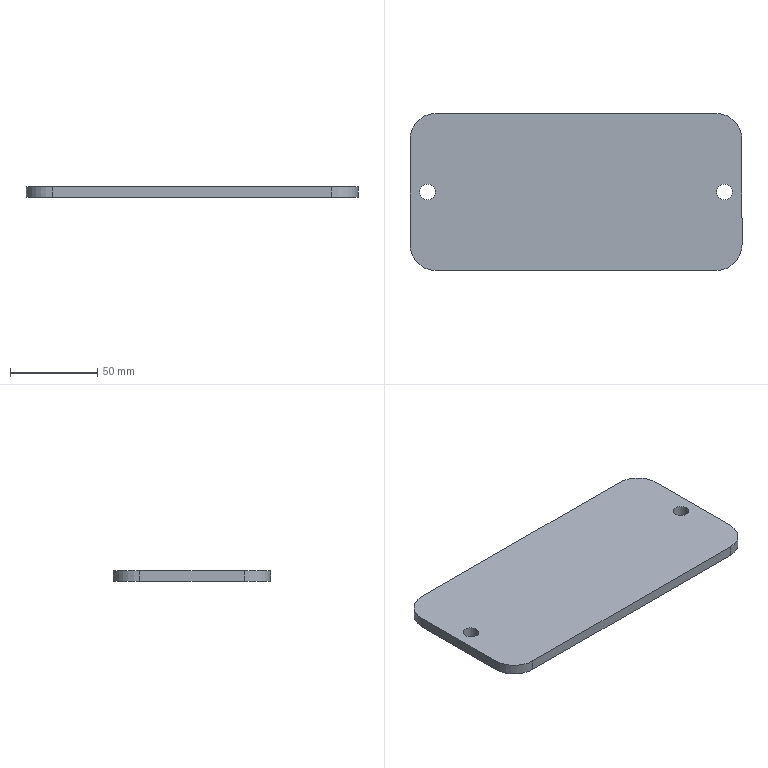Part | SolidWorks | features FlatPattern 1, SMBaseFlange 1, SheetMetal 1 | 1 solid | 14 faces | box 190 x 90 x 6 mm | volume 100678 mm3 | cylinder 8 | plane 6 | commonest cylinder face diameters 9 x4 30 x4
STEP:
#1=CARTESIAN_POINT('',(175.5,45.,-6.));
#2=VERTEX_POINT('',#1);
#3=CARTESIAN_POINT('',(184.5,45.,-6.));
#4=VERTEX_POINT('',#3);
#5=CARTESIAN_POINT('',(180.,45.,-6.));
#6=DIRECTION('',(0.,0.,1.));
#7=DIRECTION('',(1.,0.,0.));
#8=AXIS2_PLACEMENT_3D('',#5,#6,#7);
#9=CIRCLE('',#8,4.5);
#10=EDGE_CURVE('',#2,#4,#9,.T.);
#11=ORIENTED_EDGE('',*,*,#10,.F.);
#12=CARTESIAN_POINT('',(175.5,45.,0.));
#13=VERTEX_POINT('',#12);
#14=CARTESIAN_POINT('',(175.5,45.,-6.));
#15=DIRECTION('',(0.,0.,1.));
#16=VECTOR('',#15,1000.);
#17=LINE('',#14,#16);
#18=EDGE_CURVE('',#2,#13,#17,.T.);
#19=ORIENTED_EDGE('',*,*,#18,.T.);
#20=CARTESIAN_POINT('',(184.5,45.,0.));
#21=VERTEX_POINT('',#20);
#22=CARTESIAN_POINT('',(180.,45.,0.));
#23=DIRECTION('',(0.,0.,1.));
#24=DIRECTION('',(1.,0.,0.));
#25=AXIS2_PLACEMENT_3D('',#22,#23,#24);
#26=CIRCLE('',#25,4.5);
#27=EDGE_CURVE('',#13,#21,#26,.T.);
#28=ORIENTED_EDGE('',*,*,#27,.T.);
#29=CARTESIAN_POINT('',(184.5,45.,-6.));
#30=DIRECTION('',(0.,0.,1.));
#31=VECTOR('',#30,1000.);
#32=LINE('',#29,#31);
#33=EDGE_CURVE('',#4,#21,#32,.T.);
#34=ORIENTED_EDGE('',*,*,#33,.F.);
#35=EDGE_LOOP('',(#11,#19,#28,#34));
#36=FACE_OUTER_BOUND('',#35,.T.);
#37=CARTESIAN_POINT('',(180.,45.,-6.));
#38=DIRECTION('',(0.,0.,1.));
#39=DIRECTION('',(1.,0.,0.));
#40=AXIS2_PLACEMENT_3D('',#37,#38,#39);
#41=CYLINDRICAL_SURFACE('',#40,4.5);
#42=ADVANCED_FACE('',(#36),#41,.F.);
#43=CARTESIAN_POINT('',(5.5,45.,-6.));
#44=VERTEX_POINT('',#43);
#45=CARTESIAN_POINT('',(14.5,45.,-6.));
#46=VERTEX_POINT('',#45);
#47=CARTESIAN_POINT('',(10.,45.,-6.));
#48=DIRECTION('',(0.,0.,1.));
#49=DIRECTION('',(1.,0.,0.));
#50=AXIS2_PLACEMENT_3D('',#47,#48,#49);
#51=CIRCLE('',#50,4.5);
#52=EDGE_CURVE('',#44,#46,#51,.T.);
#53=ORIENTED_EDGE('',*,*,#52,.F.);
#54=CARTESIAN_POINT('',(5.5,45.,0.));
#55=VERTEX_POINT('',#54);
#56=CARTESIAN_POINT('',(5.5,45.,-6.));
#57=DIRECTION('',(0.,0.,1.));
#58=VECTOR('',#57,1000.);
#59=LINE('',#56,#58);
#60=EDGE_CURVE('',#44,#55,#59,.T.);
#61=ORIENTED_EDGE('',*,*,#60,.T.);
#62=CARTESIAN_POINT('',(14.5,45.,0.));
#63=VERTEX_POINT('',#62);
#64=CARTESIAN_POINT('',(10.,45.,0.));
#65=DIRECTION('',(0.,0.,1.));
#66=DIRECTION('',(1.,0.,0.));
#67=AXIS2_PLACEMENT_3D('',#64,#65,#66);
#68=CIRCLE('',#67,4.5);
#69=EDGE_CURVE('',#55,#63,#68,.T.);
#70=ORIENTED_EDGE('',*,*,#69,.T.);
#71=CARTESIAN_POINT('',(14.5,45.,-6.));
#72=DIRECTION('',(0.,0.,1.));
#73=VECTOR('',#72,1000.);
#74=LINE('',#71,#73);
#75=EDGE_CURVE('',#46,#63,#74,.T.);
#76=ORIENTED_EDGE('',*,*,#75,.F.);
#77=EDGE_LOOP('',(#53,#61,#70,#76));
#78=FACE_OUTER_BOUND('',#77,.T.);
#79=CARTESIAN_POINT('',(10.,45.,-6.));
#80=DIRECTION('',(0.,0.,1.));
#81=DIRECTION('',(1.,0.,0.));
#82=AXIS2_PLACEMENT_3D('',#79,#80,#81);
#83=CYLINDRICAL_SURFACE('',#82,4.5);
#84=ADVANCED_FACE('',(#78),#83,.F.);
#85=CARTESIAN_POINT('',(175.,0.,0.));
#86=VERTEX_POINT('',#85);
#87=CARTESIAN_POINT('',(190.,15.,0.));
#88=VERTEX_POINT('',#87);
#89=CARTESIAN_POINT('',(175.,15.,0.));
#90=DIRECTION('',(0.,0.,1.));
#91=DIRECTION('',(-1.,0.,0.));
#92=AXIS2_PLACEMENT_3D('',#89,#90,#91);
#93=CIRCLE('',#92,15.);
#94=EDGE_CURVE('',#86,#88,#93,.T.);
#95=ORIENTED_EDGE('',*,*,#94,.F.);
#96=CARTESIAN_POINT('',(175.,0.,-6.));
#97=VERTEX_POINT('',#96);
#98=CARTESIAN_POINT('',(175.,0.,-6.));
#99=DIRECTION('',(0.,0.,1.));
#100=VECTOR('',#99,1000.);
#101=LINE('',#98,#100);
#102=EDGE_CURVE('',#97,#86,#101,.T.);
#103=ORIENTED_EDGE('',*,*,#102,.F.);
#104=CARTESIAN_POINT('',(190.,15.,-6.));
#105=VERTEX_POINT('',#104);
#106=CARTESIAN_POINT('',(175.,15.,-6.));
#107=DIRECTION('',(0.,0.,1.));
#108=DIRECTION('',(-1.,0.,0.));
#109=AXIS2_PLACEMENT_3D('',#106,#107,#108);
#110=CIRCLE('',#109,15.);
#111=EDGE_CURVE('',#97,#105,#110,.T.);
#112=ORIENTED_EDGE('',*,*,#111,.T.);
#113=CARTESIAN_POINT('',(190.,15.,-6.));
#114=DIRECTION('',(0.,0.,1.));
#115=VECTOR('',#114,1000.);
#116=LINE('',#113,#115);
#117=EDGE_CURVE('',#105,#88,#116,.T.);
#118=ORIENTED_EDGE('',*,*,#117,.T.);
#119=EDGE_LOOP('',(#95,#103,#112,#118));
#120=FACE_OUTER_BOUND('',#119,.T.);
#121=CARTESIAN_POINT('',(175.,15.,-6.));
#122=DIRECTION('',(0.,0.,1.));
#123=DIRECTION('',(1.,0.,0.));
#124=AXIS2_PLACEMENT_3D('',#121,#122,#123);
#125=CYLINDRICAL_SURFACE('',#124,15.);
#126=ADVANCED_FACE('',(#120),#125,.T.);
#127=CARTESIAN_POINT('',(15.,0.,0.));
#128=VERTEX_POINT('',#127);
#129=CARTESIAN_POINT('',(15.,0.,0.));
#130=DIRECTION('',(1.,0.,0.));
#131=VECTOR('',#130,1000.);
#132=LINE('',#129,#131);
#133=EDGE_CURVE('',#128,#86,#132,.T.);
#134=ORIENTED_EDGE('',*,*,#133,.F.);
#135=CARTESIAN_POINT('',(15.,0.,-6.));
#136=VERTEX_POINT('',#135);
#137=CARTESIAN_POINT('',(15.,0.,-6.));
#138=DIRECTION('',(0.,0.,1.));
#139=VECTOR('',#138,1000.);
#140=LINE('',#137,#139);
#141=EDGE_CURVE('',#136,#128,#140,.T.);
#142=ORIENTED_EDGE('',*,*,#141,.F.);
#143=CARTESIAN_POINT('',(15.,0.,-6.));
#144=DIRECTION('',(1.,0.,0.));
#145=VECTOR('',#144,1000.);
#146=LINE('',#143,#145);
#147=EDGE_CURVE('',#136,#97,#146,.T.);
#148=ORIENTED_EDGE('',*,*,#147,.T.);
#149=ORIENTED_EDGE('',*,*,#102,.T.);
#150=EDGE_LOOP('',(#134,#142,#148,#149));
#151=FACE_OUTER_BOUND('',#150,.T.);
#152=CARTESIAN_POINT('',(15.,0.,-6.));
#153=DIRECTION('',(0.,-1.,0.));
#154=DIRECTION('',(0.,0.,-1.));
#155=AXIS2_PLACEMENT_3D('',#152,#153,#154);
#156=PLANE('',#155);
#157=ADVANCED_FACE('',(#151),#156,.T.);
#158=CARTESIAN_POINT('',(0.,15.,0.));
#159=VERTEX_POINT('',#158);
#160=CARTESIAN_POINT('',(15.,15.,0.));
#161=DIRECTION('',(0.,0.,1.));
#162=DIRECTION('',(-1.,0.,0.));
#163=AXIS2_PLACEMENT_3D('',#160,#161,#162);
#164=CIRCLE('',#163,15.);
#165=EDGE_CURVE('',#159,#128,#164,.T.);
#166=ORIENTED_EDGE('',*,*,#165,.F.);
#167=CARTESIAN_POINT('',(0.,15.,-6.));
#168=VERTEX_POINT('',#167);
#169=CARTESIAN_POINT('',(0.,15.,-6.));
#170=DIRECTION('',(0.,0.,1.));
#171=VECTOR('',#170,1000.);
#172=LINE('',#169,#171);
#173=EDGE_CURVE('',#168,#159,#172,.T.);
#174=ORIENTED_EDGE('',*,*,#173,.F.);
#175=CARTESIAN_POINT('',(15.,15.,-6.));
#176=DIRECTION('',(0.,0.,1.));
#177=DIRECTION('',(-1.,0.,0.));
#178=AXIS2_PLACEMENT_3D('',#175,#176,#177);
#179=CIRCLE('',#178,15.);
#180=EDGE_CURVE('',#168,#136,#179,.T.);
#181=ORIENTED_EDGE('',*,*,#180,.T.);
#182=ORIENTED_EDGE('',*,*,#141,.T.);
#183=EDGE_LOOP('',(#166,#174,#181,#182));
#184=FACE_OUTER_BOUND('',#183,.T.);
#185=CARTESIAN_POINT('',(15.,15.,-6.));
#186=DIRECTION('',(0.,0.,1.));
#187=DIRECTION('',(1.,0.,0.));
#188=AXIS2_PLACEMENT_3D('',#185,#186,#187);
#189=CYLINDRICAL_SURFACE('',#188,15.);
#190=ADVANCED_FACE('',(#184),#189,.T.);
#191=CARTESIAN_POINT('',(0.,75.,0.));
#192=VERTEX_POINT('',#191);
#193=CARTESIAN_POINT('',(0.,15.,0.));
#194=DIRECTION('',(0.,-1.,0.));
#195=VECTOR('',#194,1000.);
#196=LINE('',#193,#195);
#197=EDGE_CURVE('',#192,#159,#196,.T.);
#198=ORIENTED_EDGE('',*,*,#197,.F.);
#199=CARTESIAN_POINT('',(0.,75.,-6.));
#200=VERTEX_POINT('',#199);
#201=CARTESIAN_POINT('',(0.,75.,-6.));
#202=DIRECTION('',(0.,0.,1.));
#203=VECTOR('',#202,1000.);
#204=LINE('',#201,#203);
#205=EDGE_CURVE('',#200,#192,#204,.T.);
#206=ORIENTED_EDGE('',*,*,#205,.F.);
#207=CARTESIAN_POINT('',(0.,15.,-6.));
#208=DIRECTION('',(0.,-1.,0.));
#209=VECTOR('',#208,1000.);
#210=LINE('',#207,#209);
#211=EDGE_CURVE('',#200,#168,#210,.T.);
#212=ORIENTED_EDGE('',*,*,#211,.T.);
#213=ORIENTED_EDGE('',*,*,#173,.T.);
#214=EDGE_LOOP('',(#198,#206,#212,#213));
#215=FACE_OUTER_BOUND('',#214,.T.);
#216=CARTESIAN_POINT('',(0.,15.,-6.));
#217=DIRECTION('',(-1.,0.,0.));
#218=DIRECTION('',(0.,-1.,0.));
#219=AXIS2_PLACEMENT_3D('',#216,#217,#218);
#220=PLANE('',#219);
#221=ADVANCED_FACE('',(#215),#220,.T.);
#222=CARTESIAN_POINT('',(15.,90.,0.));
#223=VERTEX_POINT('',#222);
#224=CARTESIAN_POINT('',(15.,75.,0.));
#225=DIRECTION('',(0.,0.,1.));
#226=DIRECTION('',(1.,0.,0.));
#227=AXIS2_PLACEMENT_3D('',#224,#225,#226);
#228=CIRCLE('',#227,15.);
#229=EDGE_CURVE('',#223,#192,#228,.T.);
#230=ORIENTED_EDGE('',*,*,#229,.F.);
#231=CARTESIAN_POINT('',(15.,90.,-6.));
#232=VERTEX_POINT('',#231);
#233=CARTESIAN_POINT('',(15.,90.,-6.));
#234=DIRECTION('',(0.,0.,1.));
#235=VECTOR('',#234,1000.);
#236=LINE('',#233,#235);
#237=EDGE_CURVE('',#232,#223,#236,.T.);
#238=ORIENTED_EDGE('',*,*,#237,.F.);
#239=CARTESIAN_POINT('',(15.,75.,-6.));
#240=DIRECTION('',(0.,0.,1.));
#241=DIRECTION('',(1.,0.,0.));
#242=AXIS2_PLACEMENT_3D('',#239,#240,#241);
#243=CIRCLE('',#242,15.);
#244=EDGE_CURVE('',#232,#200,#243,.T.);
#245=ORIENTED_EDGE('',*,*,#244,.T.);
#246=ORIENTED_EDGE('',*,*,#205,.T.);
#247=EDGE_LOOP('',(#230,#238,#245,#246));
#248=FACE_OUTER_BOUND('',#247,.T.);
#249=CARTESIAN_POINT('',(15.,75.,-6.));
#250=DIRECTION('',(0.,0.,1.));
#251=DIRECTION('',(1.,0.,0.));
#252=AXIS2_PLACEMENT_3D('',#249,#250,#251);
#253=CYLINDRICAL_SURFACE('',#252,15.);
#254=ADVANCED_FACE('',(#248),#253,.T.);
#255=CARTESIAN_POINT('',(175.,90.,0.));
#256=VERTEX_POINT('',#255);
#257=CARTESIAN_POINT('',(15.,90.,0.));
#258=DIRECTION('',(-1.,0.,0.));
#259=VECTOR('',#258,1000.);
#260=LINE('',#257,#259);
#261=EDGE_CURVE('',#256,#223,#260,.T.);
#262=ORIENTED_EDGE('',*,*,#261,.F.);
#263=CARTESIAN_POINT('',(175.,90.,-6.));
#264=VERTEX_POINT('',#263);
#265=CARTESIAN_POINT('',(175.,90.,-6.));
#266=DIRECTION('',(0.,0.,1.));
#267=VECTOR('',#266,1000.);
#268=LINE('',#265,#267);
#269=EDGE_CURVE('',#264,#256,#268,.T.);
#270=ORIENTED_EDGE('',*,*,#269,.F.);
#271=CARTESIAN_POINT('',(15.,90.,-6.));
#272=DIRECTION('',(-1.,0.,0.));
#273=VECTOR('',#272,1000.);
#274=LINE('',#271,#273);
#275=EDGE_CURVE('',#264,#232,#274,.T.);
#276=ORIENTED_EDGE('',*,*,#275,.T.);
#277=ORIENTED_EDGE('',*,*,#237,.T.);
#278=EDGE_LOOP('',(#262,#270,#276,#277));
#279=FACE_OUTER_BOUND('',#278,.T.);
#280=CARTESIAN_POINT('',(15.,90.,-6.));
#281=DIRECTION('',(0.,1.,0.));
#282=DIRECTION('',(0.,0.,1.));
#283=AXIS2_PLACEMENT_3D('',#280,#281,#282);
#284=PLANE('',#283);
#285=ADVANCED_FACE('',(#279),#284,.T.);
#286=CARTESIAN_POINT('',(190.,75.,0.));
#287=VERTEX_POINT('',#286);
#288=CARTESIAN_POINT('',(175.,75.,0.));
#289=DIRECTION('',(0.,0.,1.));
#290=DIRECTION('',(1.,0.,0.));
#291=AXIS2_PLACEMENT_3D('',#288,#289,#290);
#292=CIRCLE('',#291,15.);
#293=EDGE_CURVE('',#287,#256,#292,.T.);
#294=ORIENTED_EDGE('',*,*,#293,.F.);
#295=CARTESIAN_POINT('',(190.,75.,-6.));
#296=VERTEX_POINT('',#295);
#297=CARTESIAN_POINT('',(190.,75.,-6.));
#298=DIRECTION('',(0.,0.,1.));
#299=VECTOR('',#298,1000.);
#300=LINE('',#297,#299);
#301=EDGE_CURVE('',#296,#287,#300,.T.);
#302=ORIENTED_EDGE('',*,*,#301,.F.);
#303=CARTESIAN_POINT('',(175.,75.,-6.));
#304=DIRECTION('',(0.,0.,1.));
#305=DIRECTION('',(1.,0.,0.));
#306=AXIS2_PLACEMENT_3D('',#303,#304,#305);
#307=CIRCLE('',#306,15.);
#308=EDGE_CURVE('',#296,#264,#307,.T.);
#309=ORIENTED_EDGE('',*,*,#308,.T.);
#310=ORIENTED_EDGE('',*,*,#269,.T.);
#311=EDGE_LOOP('',(#294,#302,#309,#310));
#312=FACE_OUTER_BOUND('',#311,.T.);
#313=CARTESIAN_POINT('',(175.,75.,-6.));
#314=DIRECTION('',(0.,0.,1.));
#315=DIRECTION('',(1.,0.,0.));
#316=AXIS2_PLACEMENT_3D('',#313,#314,#315);
#317=CYLINDRICAL_SURFACE('',#316,15.);
#318=ADVANCED_FACE('',(#312),#317,.T.);
#319=CARTESIAN_POINT('',(190.,15.,0.));
#320=DIRECTION('',(0.,1.,0.));
#321=VECTOR('',#320,1000.);
#322=LINE('',#319,#321);
#323=EDGE_CURVE('',#88,#287,#322,.T.);
#324=ORIENTED_EDGE('',*,*,#323,.F.);
#325=ORIENTED_EDGE('',*,*,#117,.F.);
#326=CARTESIAN_POINT('',(190.,15.,-6.));
#327=DIRECTION('',(0.,1.,0.));
#328=VECTOR('',#327,1000.);
#329=LINE('',#326,#328);
#330=EDGE_CURVE('',#105,#296,#329,.T.);
#331=ORIENTED_EDGE('',*,*,#330,.T.);
#332=ORIENTED_EDGE('',*,*,#301,.T.);
#333=EDGE_LOOP('',(#324,#325,#331,#332));
#334=FACE_OUTER_BOUND('',#333,.T.);
#335=CARTESIAN_POINT('',(190.,15.,-6.));
#336=DIRECTION('',(1.,0.,0.));
#337=DIRECTION('',(0.,1.,0.));
#338=AXIS2_PLACEMENT_3D('',#335,#336,#337);
#339=PLANE('',#338);
#340=ADVANCED_FACE('',(#334),#339,.T.);
#341=CARTESIAN_POINT('',(180.,45.,-6.));
#342=DIRECTION('',(0.,0.,1.));
#343=DIRECTION('',(1.,0.,0.));
#344=AXIS2_PLACEMENT_3D('',#341,#342,#343);
#345=CIRCLE('',#344,4.5);
#346=EDGE_CURVE('',#4,#2,#345,.T.);
#347=ORIENTED_EDGE('',*,*,#346,.T.);
#348=ORIENTED_EDGE('',*,*,#10,.T.);
#349=EDGE_LOOP('',(#347,#348));
#350=FACE_BOUND('',#349,.T.);
#351=CARTESIAN_POINT('',(10.,45.,-6.));
#352=DIRECTION('',(0.,0.,1.));
#353=DIRECTION('',(1.,0.,0.));
#354=AXIS2_PLACEMENT_3D('',#351,#352,#353);
#355=CIRCLE('',#354,4.5);
#356=EDGE_CURVE('',#46,#44,#355,.T.);
#357=ORIENTED_EDGE('',*,*,#356,.T.);
#358=ORIENTED_EDGE('',*,*,#52,.T.);
#359=EDGE_LOOP('',(#357,#358));
#360=FACE_BOUND('',#359,.T.);
#361=ORIENTED_EDGE('',*,*,#111,.F.);
#362=ORIENTED_EDGE('',*,*,#147,.F.);
#363=ORIENTED_EDGE('',*,*,#180,.F.);
#364=ORIENTED_EDGE('',*,*,#211,.F.);
#365=ORIENTED_EDGE('',*,*,#244,.F.);
#366=ORIENTED_EDGE('',*,*,#275,.F.);
#367=ORIENTED_EDGE('',*,*,#308,.F.);
#368=ORIENTED_EDGE('',*,*,#330,.F.);
#369=EDGE_LOOP('',(#361,#362,#363,#364,#365,#366,#367,#368));
#370=FACE_OUTER_BOUND('',#369,.T.);
#371=CARTESIAN_POINT('',(175.,15.,-6.));
#372=DIRECTION('',(0.,0.,-1.));
#373=DIRECTION('',(-1.,0.,0.));
#374=AXIS2_PLACEMENT_3D('',#371,#372,#373);
#375=PLANE('',#374);
#376=ADVANCED_FACE('',(#350,#360,#370),#375,.T.);
#377=CARTESIAN_POINT('',(180.,45.,0.));
#378=DIRECTION('',(0.,0.,1.));
#379=DIRECTION('',(1.,0.,0.));
#380=AXIS2_PLACEMENT_3D('',#377,#378,#379);
#381=CIRCLE('',#380,4.5);
#382=EDGE_CURVE('',#21,#13,#381,.T.);
#383=ORIENTED_EDGE('',*,*,#382,.F.);
#384=ORIENTED_EDGE('',*,*,#27,.F.);
#385=EDGE_LOOP('',(#383,#384));
#386=FACE_BOUND('',#385,.T.);
#387=CARTESIAN_POINT('',(10.,45.,0.));
#388=DIRECTION('',(0.,0.,1.));
#389=DIRECTION('',(1.,0.,0.));
#390=AXIS2_PLACEMENT_3D('',#387,#388,#389);
#391=CIRCLE('',#390,4.5);
#392=EDGE_CURVE('',#63,#55,#391,.T.);
#393=ORIENTED_EDGE('',*,*,#392,.F.);
#394=ORIENTED_EDGE('',*,*,#69,.F.);
#395=EDGE_LOOP('',(#393,#394));
#396=FACE_BOUND('',#395,.T.);
#397=ORIENTED_EDGE('',*,*,#94,.T.);
#398=ORIENTED_EDGE('',*,*,#323,.T.);
#399=ORIENTED_EDGE('',*,*,#293,.T.);
#400=ORIENTED_EDGE('',*,*,#261,.T.);
#401=ORIENTED_EDGE('',*,*,#229,.T.);
#402=ORIENTED_EDGE('',*,*,#197,.T.);
#403=ORIENTED_EDGE('',*,*,#165,.T.);
#404=ORIENTED_EDGE('',*,*,#133,.T.);
#405=EDGE_LOOP('',(#397,#398,#399,#400,#401,#402,#403,#404));
#406=FACE_OUTER_BOUND('',#405,.T.);
#407=CARTESIAN_POINT('',(175.,15.,0.));
#408=DIRECTION('',(0.,0.,-1.));
#409=DIRECTION('',(-1.,0.,0.));
#410=AXIS2_PLACEMENT_3D('',#407,#408,#409);
#411=PLANE('',#410);
#412=ADVANCED_FACE('',(#386,#396,#406),#411,.F.);
#413=ORIENTED_EDGE('',*,*,#60,.F.);
#414=ORIENTED_EDGE('',*,*,#356,.F.);
#415=ORIENTED_EDGE('',*,*,#75,.T.);
#416=ORIENTED_EDGE('',*,*,#392,.T.);
#417=EDGE_LOOP('',(#413,#414,#415,#416));
#418=FACE_OUTER_BOUND('',#417,.T.);
#419=CARTESIAN_POINT('',(10.,45.,-6.));
#420=DIRECTION('',(0.,0.,1.));
#421=DIRECTION('',(1.,0.,0.));
#422=AXIS2_PLACEMENT_3D('',#419,#420,#421);
#423=CYLINDRICAL_SURFACE('',#422,4.5);
#424=ADVANCED_FACE('',(#418),#423,.F.);
#425=ORIENTED_EDGE('',*,*,#18,.F.);
#426=ORIENTED_EDGE('',*,*,#346,.F.);
#427=ORIENTED_EDGE('',*,*,#33,.T.);
#428=ORIENTED_EDGE('',*,*,#382,.T.);
#429=EDGE_LOOP('',(#425,#426,#427,#428));
#430=FACE_OUTER_BOUND('',#429,.T.);
#431=CARTESIAN_POINT('',(180.,45.,-6.));
#432=DIRECTION('',(0.,0.,1.));
#433=DIRECTION('',(1.,0.,0.));
#434=AXIS2_PLACEMENT_3D('',#431,#432,#433);
#435=CYLINDRICAL_SURFACE('',#434,4.5);
#436=ADVANCED_FACE('',(#430),#435,.F.);
#437=CLOSED_SHELL('',(#42,#84,#126,#157,#190,#221,#254,#285,#318,#340,#376,#412,#424,#436));
#438=MANIFOLD_SOLID_BREP('',#437);
#439=CARTESIAN_POINT('',(0.,0.,0.));
#440=DIRECTION('',(0.,0.,1.));
#441=DIRECTION('',(1.,0.,0.));
#442=AXIS2_PLACEMENT_3D('',#439,#440,#441);
#443=(LENGTH_UNIT()NAMED_UNIT(*)SI_UNIT(.MILLI.,.METRE.));
#444=UNCERTAINTY_MEASURE_WITH_UNIT(LENGTH_MEASURE(0.00001),#443,'','');
#445=(NAMED_UNIT(*)PLANE_ANGLE_UNIT()SI_UNIT($,.RADIAN.));
#446=(NAMED_UNIT(*)SI_UNIT($,.STERADIAN.)SOLID_ANGLE_UNIT());
#447=(GEOMETRIC_REPRESENTATION_CONTEXT(3)GLOBAL_UNCERTAINTY_ASSIGNED_CONTEXT((#444))GLOBAL_UNIT_ASSIGNED_CONTEXT((#443,#445,#446))REPRESENTATION_CONTEXT('',''));
#448=ADVANCED_BREP_SHAPE_REPRESENTATION('',(#438,#442),#447);